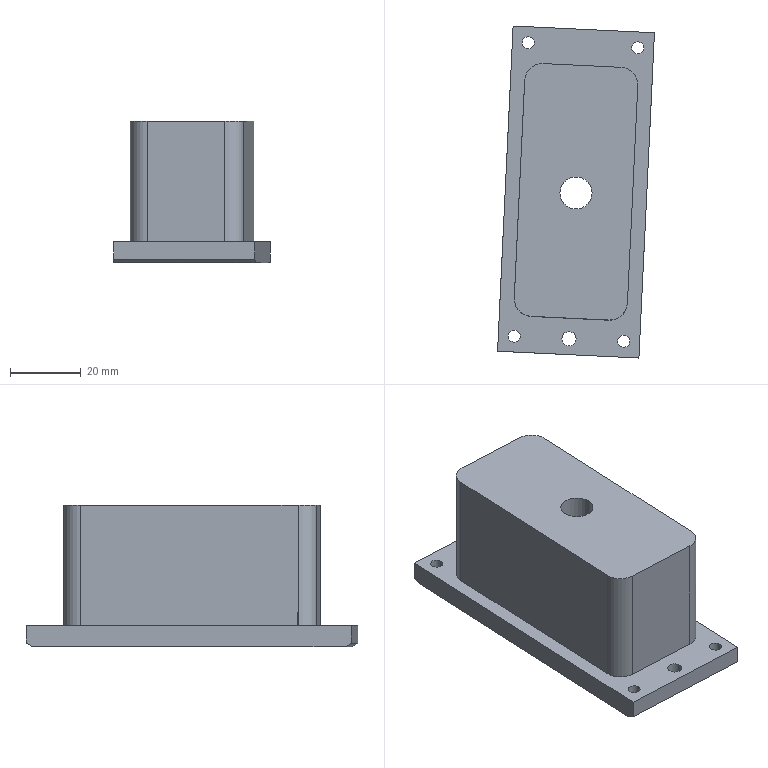Part | STEP file | X77b-08201 | 1 solid | 365 faces | box 44.351 x 93.807 x 40.034 mm | volume 61790 mm3 | cylinder 138 | plane 116 | spline 104 | cone 4 | sphere 2 | torus 1 | commonest cylinder face diameters 1 x81 4 x14 0.8 x10 6 x9 3.4 x8 10 x5